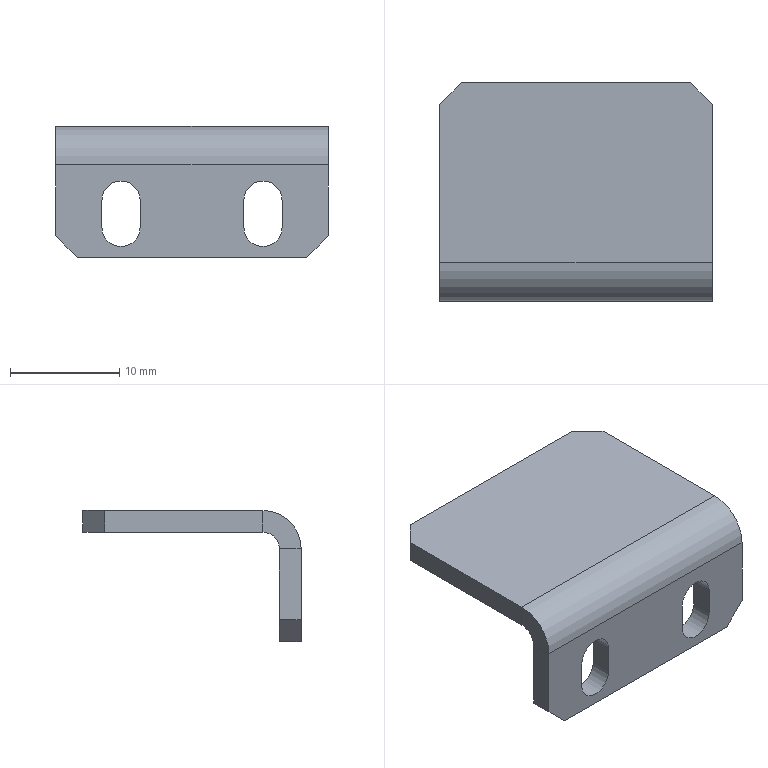Part | STEP file | 227H056379 BKT_Default | 1 solid | 28 faces | box 25 x 20 x 12 mm | volume 1357 mm3 | plane 20 | cylinder 8 | commonest cylinder face diameters 3.5 x6 3 x1 7 x1